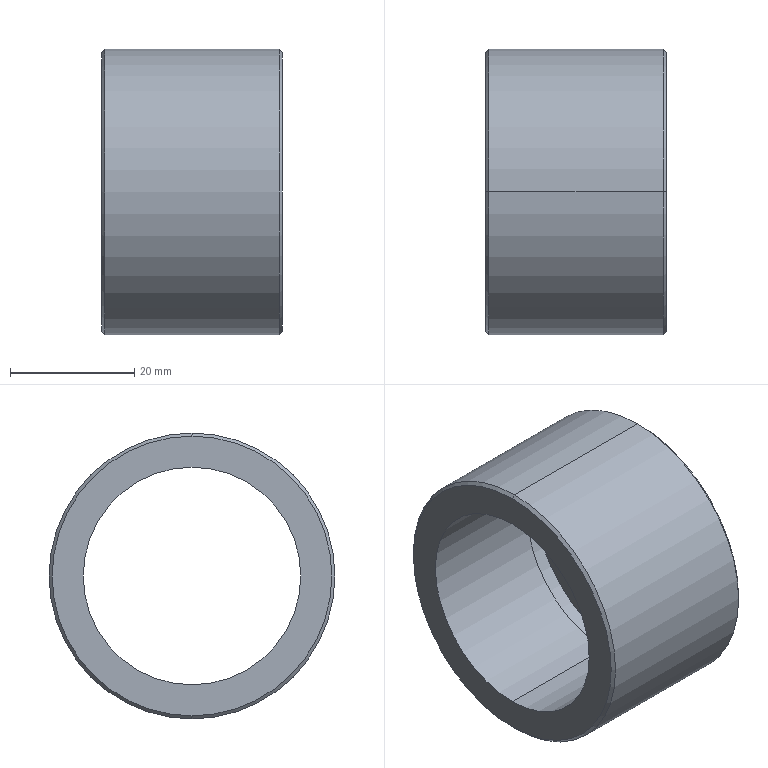Part | SolidWorks | features Chamfer 1, Revolution 1 | 1 solid | 16 faces | box 29 x 46 x 46 mm | volume 17975 mm3 | cylinder 8 | cone 4 | plane 4 | commonest cylinder face diameters 35 x4 42.5 x2 46 x2
STEP:
#1=CARTESIAN_POINT('',(0.,0.,22.5));
#2=VERTEX_POINT('',#1);
#3=CARTESIAN_POINT('',(0.,0.,-22.5));
#4=VERTEX_POINT('',#3);
#5=CARTESIAN_POINT('',(0.,0.,0.));
#6=DIRECTION('',(-1.,0.,0.));
#7=DIRECTION('',(0.,0.,-1.));
#8=AXIS2_PLACEMENT_3D('',#5,#6,#7);
#9=CIRCLE('',#8,22.5);
#10=EDGE_CURVE('',#2,#4,#9,.T.);
#11=ORIENTED_EDGE('',*,*,#10,.F.);
#12=CARTESIAN_POINT('',(0.5,0.,23.));
#13=VERTEX_POINT('',#12);
#14=CARTESIAN_POINT('',(0.,0.,22.5));
#15=DIRECTION('',(0.7071,0.,0.7071));
#16=VECTOR('',#15,1000.);
#17=LINE('',#14,#16);
#18=EDGE_CURVE('',#2,#13,#17,.T.);
#19=ORIENTED_EDGE('',*,*,#18,.T.);
#20=CARTESIAN_POINT('',(0.5,0.,-23.));
#21=VERTEX_POINT('',#20);
#22=CARTESIAN_POINT('',(0.5,0.,0.));
#23=DIRECTION('',(1.,0.,0.));
#24=DIRECTION('',(0.,0.,-1.));
#25=AXIS2_PLACEMENT_3D('',#22,#23,#24);
#26=CIRCLE('',#25,23.);
#27=EDGE_CURVE('',#21,#13,#26,.T.);
#28=ORIENTED_EDGE('',*,*,#27,.F.);
#29=CARTESIAN_POINT('',(0.,0.,-22.5));
#30=DIRECTION('',(0.7071,0.,-0.7071));
#31=VECTOR('',#30,1000.);
#32=LINE('',#29,#31);
#33=EDGE_CURVE('',#4,#21,#32,.T.);
#34=ORIENTED_EDGE('',*,*,#33,.F.);
#35=EDGE_LOOP('',(#11,#19,#28,#34));
#36=FACE_OUTER_BOUND('',#35,.T.);
#37=CARTESIAN_POINT('',(0.,0.,0.));
#38=DIRECTION('',(1.,0.,0.));
#39=DIRECTION('',(0.,0.,-1.));
#40=AXIS2_PLACEMENT_3D('',#37,#38,#39);
#41=CONICAL_SURFACE('',#40,22.5,0.7854);
#42=ADVANCED_FACE('',(#36),#41,.T.);
#43=CARTESIAN_POINT('',(29.,0.,-22.5));
#44=VERTEX_POINT('',#43);
#45=CARTESIAN_POINT('',(29.,0.,22.5));
#46=VERTEX_POINT('',#45);
#47=CARTESIAN_POINT('',(29.,0.,0.));
#48=DIRECTION('',(1.,0.,0.));
#49=DIRECTION('',(0.,0.,1.));
#50=AXIS2_PLACEMENT_3D('',#47,#48,#49);
#51=CIRCLE('',#50,22.5);
#52=EDGE_CURVE('',#44,#46,#51,.T.);
#53=ORIENTED_EDGE('',*,*,#52,.F.);
#54=CARTESIAN_POINT('',(28.5,0.,-23.));
#55=VERTEX_POINT('',#54);
#56=CARTESIAN_POINT('',(28.5,0.,-23.));
#57=DIRECTION('',(-0.7071,0.,-0.7071));
#58=VECTOR('',#57,1000.);
#59=LINE('',#56,#58);
#60=EDGE_CURVE('',#44,#55,#59,.T.);
#61=ORIENTED_EDGE('',*,*,#60,.T.);
#62=CARTESIAN_POINT('',(28.5,0.,23.));
#63=VERTEX_POINT('',#62);
#64=CARTESIAN_POINT('',(28.5,0.,0.));
#65=DIRECTION('',(-1.,0.,0.));
#66=DIRECTION('',(0.,0.,1.));
#67=AXIS2_PLACEMENT_3D('',#64,#65,#66);
#68=CIRCLE('',#67,23.);
#69=EDGE_CURVE('',#63,#55,#68,.T.);
#70=ORIENTED_EDGE('',*,*,#69,.F.);
#71=CARTESIAN_POINT('',(28.5,0.,23.));
#72=DIRECTION('',(-0.7071,0.,0.7071));
#73=VECTOR('',#72,1000.);
#74=LINE('',#71,#73);
#75=EDGE_CURVE('',#46,#63,#74,.T.);
#76=ORIENTED_EDGE('',*,*,#75,.F.);
#77=EDGE_LOOP('',(#53,#61,#70,#76));
#78=FACE_OUTER_BOUND('',#77,.T.);
#79=CARTESIAN_POINT('',(28.5,0.,0.));
#80=DIRECTION('',(-1.,0.,0.));
#81=DIRECTION('',(0.,0.,1.));
#82=AXIS2_PLACEMENT_3D('',#79,#80,#81);
#83=CONICAL_SURFACE('',#82,23.,0.7854);
#84=ADVANCED_FACE('',(#78),#83,.T.);
#85=CARTESIAN_POINT('',(21.,0.,-17.5));
#86=VERTEX_POINT('',#85);
#87=CARTESIAN_POINT('',(21.,0.,17.5));
#88=VERTEX_POINT('',#87);
#89=CARTESIAN_POINT('',(21.,0.,0.));
#90=DIRECTION('',(-1.,0.,0.));
#91=DIRECTION('',(0.,0.,1.));
#92=AXIS2_PLACEMENT_3D('',#89,#90,#91);
#93=CIRCLE('',#92,17.5);
#94=EDGE_CURVE('',#86,#88,#93,.T.);
#95=ORIENTED_EDGE('',*,*,#94,.F.);
#96=CARTESIAN_POINT('',(0.,0.,-17.5));
#97=VERTEX_POINT('',#96);
#98=CARTESIAN_POINT('',(0.,0.,-17.5));
#99=DIRECTION('',(-1.,0.,0.));
#100=VECTOR('',#99,1000.);
#101=LINE('',#98,#100);
#102=EDGE_CURVE('',#86,#97,#101,.T.);
#103=ORIENTED_EDGE('',*,*,#102,.T.);
#104=CARTESIAN_POINT('',(0.,0.,17.5));
#105=VERTEX_POINT('',#104);
#106=CARTESIAN_POINT('',(0.,0.,0.));
#107=DIRECTION('',(-1.,0.,0.));
#108=DIRECTION('',(0.,0.,1.));
#109=AXIS2_PLACEMENT_3D('',#106,#107,#108);
#110=CIRCLE('',#109,17.5);
#111=EDGE_CURVE('',#97,#105,#110,.T.);
#112=ORIENTED_EDGE('',*,*,#111,.T.);
#113=CARTESIAN_POINT('',(0.,0.,17.5));
#114=DIRECTION('',(-1.,0.,0.));
#115=VECTOR('',#114,1000.);
#116=LINE('',#113,#115);
#117=EDGE_CURVE('',#88,#105,#116,.T.);
#118=ORIENTED_EDGE('',*,*,#117,.F.);
#119=EDGE_LOOP('',(#95,#103,#112,#118));
#120=FACE_OUTER_BOUND('',#119,.T.);
#121=CARTESIAN_POINT('',(0.,0.,0.));
#122=DIRECTION('',(-1.,0.,0.));
#123=DIRECTION('',(0.,0.,1.));
#124=AXIS2_PLACEMENT_3D('',#121,#122,#123);
#125=CYLINDRICAL_SURFACE('',#124,17.5);
#126=ADVANCED_FACE('',(#120),#125,.F.);
#127=CARTESIAN_POINT('',(26.,0.,-21.25));
#128=VERTEX_POINT('',#127);
#129=CARTESIAN_POINT('',(26.,0.,21.25));
#130=VERTEX_POINT('',#129);
#131=CARTESIAN_POINT('',(26.,0.,0.));
#132=DIRECTION('',(-1.,0.,0.));
#133=DIRECTION('',(0.,0.,1.));
#134=AXIS2_PLACEMENT_3D('',#131,#132,#133);
#135=CIRCLE('',#134,21.25);
#136=EDGE_CURVE('',#128,#130,#135,.T.);
#137=ORIENTED_EDGE('',*,*,#136,.F.);
#138=CARTESIAN_POINT('',(21.,0.,-21.25));
#139=VERTEX_POINT('',#138);
#140=CARTESIAN_POINT('',(0.,0.,-21.25));
#141=DIRECTION('',(-1.,0.,0.));
#142=VECTOR('',#141,1000.);
#143=LINE('',#140,#142);
#144=EDGE_CURVE('',#128,#139,#143,.T.);
#145=ORIENTED_EDGE('',*,*,#144,.T.);
#146=CARTESIAN_POINT('',(21.,0.,21.25));
#147=VERTEX_POINT('',#146);
#148=CARTESIAN_POINT('',(21.,0.,0.));
#149=DIRECTION('',(-1.,0.,0.));
#150=DIRECTION('',(0.,0.,1.));
#151=AXIS2_PLACEMENT_3D('',#148,#149,#150);
#152=CIRCLE('',#151,21.25);
#153=EDGE_CURVE('',#139,#147,#152,.T.);
#154=ORIENTED_EDGE('',*,*,#153,.T.);
#155=CARTESIAN_POINT('',(0.,0.,21.25));
#156=DIRECTION('',(-1.,0.,0.));
#157=VECTOR('',#156,1000.);
#158=LINE('',#155,#157);
#159=EDGE_CURVE('',#130,#147,#158,.T.);
#160=ORIENTED_EDGE('',*,*,#159,.F.);
#161=EDGE_LOOP('',(#137,#145,#154,#160));
#162=FACE_OUTER_BOUND('',#161,.T.);
#163=CARTESIAN_POINT('',(0.,0.,0.));
#164=DIRECTION('',(-1.,0.,0.));
#165=DIRECTION('',(0.,0.,1.));
#166=AXIS2_PLACEMENT_3D('',#163,#164,#165);
#167=CYLINDRICAL_SURFACE('',#166,21.25);
#168=ADVANCED_FACE('',(#162),#167,.F.);
#169=CARTESIAN_POINT('',(29.,0.,-17.5));
#170=VERTEX_POINT('',#169);
#171=CARTESIAN_POINT('',(29.,0.,17.5));
#172=VERTEX_POINT('',#171);
#173=CARTESIAN_POINT('',(29.,0.,0.));
#174=DIRECTION('',(-1.,0.,0.));
#175=DIRECTION('',(0.,0.,1.));
#176=AXIS2_PLACEMENT_3D('',#173,#174,#175);
#177=CIRCLE('',#176,17.5);
#178=EDGE_CURVE('',#170,#172,#177,.T.);
#179=ORIENTED_EDGE('',*,*,#178,.F.);
#180=CARTESIAN_POINT('',(26.,0.,-17.5));
#181=VERTEX_POINT('',#180);
#182=CARTESIAN_POINT('',(0.,0.,-17.5));
#183=DIRECTION('',(-1.,0.,0.));
#184=VECTOR('',#183,1000.);
#185=LINE('',#182,#184);
#186=EDGE_CURVE('',#170,#181,#185,.T.);
#187=ORIENTED_EDGE('',*,*,#186,.T.);
#188=CARTESIAN_POINT('',(26.,0.,17.5));
#189=VERTEX_POINT('',#188);
#190=CARTESIAN_POINT('',(26.,0.,0.));
#191=DIRECTION('',(-1.,0.,0.));
#192=DIRECTION('',(0.,0.,1.));
#193=AXIS2_PLACEMENT_3D('',#190,#191,#192);
#194=CIRCLE('',#193,17.5);
#195=EDGE_CURVE('',#181,#189,#194,.T.);
#196=ORIENTED_EDGE('',*,*,#195,.T.);
#197=CARTESIAN_POINT('',(0.,0.,17.5));
#198=DIRECTION('',(-1.,0.,0.));
#199=VECTOR('',#198,1000.);
#200=LINE('',#197,#199);
#201=EDGE_CURVE('',#172,#189,#200,.T.);
#202=ORIENTED_EDGE('',*,*,#201,.F.);
#203=EDGE_LOOP('',(#179,#187,#196,#202));
#204=FACE_OUTER_BOUND('',#203,.T.);
#205=CARTESIAN_POINT('',(0.,0.,0.));
#206=DIRECTION('',(-1.,0.,0.));
#207=DIRECTION('',(0.,0.,1.));
#208=AXIS2_PLACEMENT_3D('',#205,#206,#207);
#209=CYLINDRICAL_SURFACE('',#208,17.5);
#210=ADVANCED_FACE('',(#204),#209,.F.);
#211=ORIENTED_EDGE('',*,*,#69,.T.);
#212=CARTESIAN_POINT('',(0.,0.,-23.));
#213=DIRECTION('',(-1.,0.,0.));
#214=VECTOR('',#213,1000.);
#215=LINE('',#212,#214);
#216=EDGE_CURVE('',#55,#21,#215,.T.);
#217=ORIENTED_EDGE('',*,*,#216,.T.);
#218=ORIENTED_EDGE('',*,*,#27,.T.);
#219=CARTESIAN_POINT('',(0.,0.,23.));
#220=DIRECTION('',(-1.,0.,0.));
#221=VECTOR('',#220,1000.);
#222=LINE('',#219,#221);
#223=EDGE_CURVE('',#63,#13,#222,.T.);
#224=ORIENTED_EDGE('',*,*,#223,.F.);
#225=EDGE_LOOP('',(#211,#217,#218,#224));
#226=FACE_OUTER_BOUND('',#225,.T.);
#227=CARTESIAN_POINT('',(0.,0.,0.));
#228=DIRECTION('',(-1.,0.,0.));
#229=DIRECTION('',(0.,0.,1.));
#230=AXIS2_PLACEMENT_3D('',#227,#228,#229);
#231=CYLINDRICAL_SURFACE('',#230,23.);
#232=ADVANCED_FACE('',(#226),#231,.T.);
#233=CARTESIAN_POINT('',(0.,0.,0.));
#234=DIRECTION('',(-1.,0.,0.));
#235=DIRECTION('',(0.,0.,-1.));
#236=AXIS2_PLACEMENT_3D('',#233,#234,#235);
#237=CIRCLE('',#236,22.5);
#238=EDGE_CURVE('',#4,#2,#237,.T.);
#239=ORIENTED_EDGE('',*,*,#238,.T.);
#240=ORIENTED_EDGE('',*,*,#10,.T.);
#241=EDGE_LOOP('',(#239,#240));
#242=FACE_OUTER_BOUND('',#241,.T.);
#243=CARTESIAN_POINT('',(0.,0.,0.));
#244=DIRECTION('',(-1.,0.,0.));
#245=DIRECTION('',(0.,0.,1.));
#246=AXIS2_PLACEMENT_3D('',#243,#244,#245);
#247=CIRCLE('',#246,17.5);
#248=EDGE_CURVE('',#105,#97,#247,.T.);
#249=ORIENTED_EDGE('',*,*,#248,.F.);
#250=ORIENTED_EDGE('',*,*,#111,.F.);
#251=EDGE_LOOP('',(#249,#250));
#252=FACE_BOUND('',#251,.T.);
#253=CARTESIAN_POINT('',(0.,17.5,0.));
#254=DIRECTION('',(1.,0.,0.));
#255=DIRECTION('',(0.,0.,-1.));
#256=AXIS2_PLACEMENT_3D('',#253,#254,#255);
#257=PLANE('',#256);
#258=ADVANCED_FACE('',(#242,#252),#257,.F.);
#259=ORIENTED_EDGE('',*,*,#216,.F.);
#260=CARTESIAN_POINT('',(28.5,0.,0.));
#261=DIRECTION('',(-1.,0.,0.));
#262=DIRECTION('',(0.,0.,1.));
#263=AXIS2_PLACEMENT_3D('',#260,#261,#262);
#264=CIRCLE('',#263,23.);
#265=EDGE_CURVE('',#55,#63,#264,.T.);
#266=ORIENTED_EDGE('',*,*,#265,.T.);
#267=ORIENTED_EDGE('',*,*,#223,.T.);
#268=CARTESIAN_POINT('',(0.5,0.,0.));
#269=DIRECTION('',(1.,0.,0.));
#270=DIRECTION('',(0.,0.,-1.));
#271=AXIS2_PLACEMENT_3D('',#268,#269,#270);
#272=CIRCLE('',#271,23.);
#273=EDGE_CURVE('',#13,#21,#272,.T.);
#274=ORIENTED_EDGE('',*,*,#273,.T.);
#275=EDGE_LOOP('',(#259,#266,#267,#274));
#276=FACE_OUTER_BOUND('',#275,.T.);
#277=CARTESIAN_POINT('',(0.,0.,0.));
#278=DIRECTION('',(-1.,0.,0.));
#279=DIRECTION('',(0.,0.,1.));
#280=AXIS2_PLACEMENT_3D('',#277,#278,#279);
#281=CYLINDRICAL_SURFACE('',#280,23.);
#282=ADVANCED_FACE('',(#276),#281,.T.);
#283=CARTESIAN_POINT('',(29.,0.,0.));
#284=DIRECTION('',(1.,0.,0.));
#285=DIRECTION('',(0.,0.,1.));
#286=AXIS2_PLACEMENT_3D('',#283,#284,#285);
#287=CIRCLE('',#286,22.5);
#288=EDGE_CURVE('',#46,#44,#287,.T.);
#289=ORIENTED_EDGE('',*,*,#288,.T.);
#290=ORIENTED_EDGE('',*,*,#52,.T.);
#291=EDGE_LOOP('',(#289,#290));
#292=FACE_OUTER_BOUND('',#291,.T.);
#293=CARTESIAN_POINT('',(29.,0.,0.));
#294=DIRECTION('',(-1.,0.,0.));
#295=DIRECTION('',(0.,0.,1.));
#296=AXIS2_PLACEMENT_3D('',#293,#294,#295);
#297=CIRCLE('',#296,17.5);
#298=EDGE_CURVE('',#172,#170,#297,.T.);
#299=ORIENTED_EDGE('',*,*,#298,.T.);
#300=ORIENTED_EDGE('',*,*,#178,.T.);
#301=EDGE_LOOP('',(#299,#300));
#302=FACE_BOUND('',#301,.T.);
#303=CARTESIAN_POINT('',(29.,17.5,0.));
#304=DIRECTION('',(-1.,0.,0.));
#305=DIRECTION('',(0.,0.,1.));
#306=AXIS2_PLACEMENT_3D('',#303,#304,#305);
#307=PLANE('',#306);
#308=ADVANCED_FACE('',(#292,#302),#307,.F.);
#309=ORIENTED_EDGE('',*,*,#186,.F.);
#310=ORIENTED_EDGE('',*,*,#298,.F.);
#311=ORIENTED_EDGE('',*,*,#201,.T.);
#312=CARTESIAN_POINT('',(26.,0.,0.));
#313=DIRECTION('',(-1.,0.,0.));
#314=DIRECTION('',(0.,0.,1.));
#315=AXIS2_PLACEMENT_3D('',#312,#313,#314);
#316=CIRCLE('',#315,17.5);
#317=EDGE_CURVE('',#189,#181,#316,.T.);
#318=ORIENTED_EDGE('',*,*,#317,.T.);
#319=EDGE_LOOP('',(#309,#310,#311,#318));
#320=FACE_OUTER_BOUND('',#319,.T.);
#321=CARTESIAN_POINT('',(0.,0.,0.));
#322=DIRECTION('',(-1.,0.,0.));
#323=DIRECTION('',(0.,0.,1.));
#324=AXIS2_PLACEMENT_3D('',#321,#322,#323);
#325=CYLINDRICAL_SURFACE('',#324,17.5);
#326=ADVANCED_FACE('',(#320),#325,.F.);
#327=ORIENTED_EDGE('',*,*,#317,.F.);
#328=ORIENTED_EDGE('',*,*,#195,.F.);
#329=EDGE_LOOP('',(#327,#328));
#330=FACE_BOUND('',#329,.T.);
#331=CARTESIAN_POINT('',(26.,0.,0.));
#332=DIRECTION('',(-1.,0.,0.));
#333=DIRECTION('',(0.,0.,1.));
#334=AXIS2_PLACEMENT_3D('',#331,#332,#333);
#335=CIRCLE('',#334,21.25);
#336=EDGE_CURVE('',#130,#128,#335,.T.);
#337=ORIENTED_EDGE('',*,*,#336,.T.);
#338=ORIENTED_EDGE('',*,*,#136,.T.);
#339=EDGE_LOOP('',(#337,#338));
#340=FACE_OUTER_BOUND('',#339,.T.);
#341=CARTESIAN_POINT('',(26.,21.25,0.));
#342=DIRECTION('',(1.,0.,0.));
#343=DIRECTION('',(0.,0.,-1.));
#344=AXIS2_PLACEMENT_3D('',#341,#342,#343);
#345=PLANE('',#344);
#346=ADVANCED_FACE('',(#330,#340),#345,.F.);
#347=ORIENTED_EDGE('',*,*,#144,.F.);
#348=ORIENTED_EDGE('',*,*,#336,.F.);
#349=ORIENTED_EDGE('',*,*,#159,.T.);
#350=CARTESIAN_POINT('',(21.,0.,0.));
#351=DIRECTION('',(-1.,0.,0.));
#352=DIRECTION('',(0.,0.,1.));
#353=AXIS2_PLACEMENT_3D('',#350,#351,#352);
#354=CIRCLE('',#353,21.25);
#355=EDGE_CURVE('',#147,#139,#354,.T.);
#356=ORIENTED_EDGE('',*,*,#355,.T.);
#357=EDGE_LOOP('',(#347,#348,#349,#356));
#358=FACE_OUTER_BOUND('',#357,.T.);
#359=CARTESIAN_POINT('',(0.,0.,0.));
#360=DIRECTION('',(-1.,0.,0.));
#361=DIRECTION('',(0.,0.,1.));
#362=AXIS2_PLACEMENT_3D('',#359,#360,#361);
#363=CYLINDRICAL_SURFACE('',#362,21.25);
#364=ADVANCED_FACE('',(#358),#363,.F.);
#365=ORIENTED_EDGE('',*,*,#355,.F.);
#366=ORIENTED_EDGE('',*,*,#153,.F.);
#367=EDGE_LOOP('',(#365,#366));
#368=FACE_OUTER_BOUND('',#367,.T.);
#369=CARTESIAN_POINT('',(21.,0.,0.));
#370=DIRECTION('',(-1.,0.,0.));
#371=DIRECTION('',(0.,0.,1.));
#372=AXIS2_PLACEMENT_3D('',#369,#370,#371);
#373=CIRCLE('',#372,17.5);
#374=EDGE_CURVE('',#88,#86,#373,.T.);
#375=ORIENTED_EDGE('',*,*,#374,.T.);
#376=ORIENTED_EDGE('',*,*,#94,.T.);
#377=EDGE_LOOP('',(#375,#376));
#378=FACE_BOUND('',#377,.T.);
#379=CARTESIAN_POINT('',(21.,17.5,0.));
#380=DIRECTION('',(-1.,0.,0.));
#381=DIRECTION('',(0.,0.,1.));
#382=AXIS2_PLACEMENT_3D('',#379,#380,#381);
#383=PLANE('',#382);
#384=ADVANCED_FACE('',(#368,#378),#383,.F.);
#385=ORIENTED_EDGE('',*,*,#102,.F.);
#386=ORIENTED_EDGE('',*,*,#374,.F.);
#387=ORIENTED_EDGE('',*,*,#117,.T.);
#388=ORIENTED_EDGE('',*,*,#248,.T.);
#389=EDGE_LOOP('',(#385,#386,#387,#388));
#390=FACE_OUTER_BOUND('',#389,.T.);
#391=CARTESIAN_POINT('',(0.,0.,0.));
#392=DIRECTION('',(-1.,0.,0.));
#393=DIRECTION('',(0.,0.,1.));
#394=AXIS2_PLACEMENT_3D('',#391,#392,#393);
#395=CYLINDRICAL_SURFACE('',#394,17.5);
#396=ADVANCED_FACE('',(#390),#395,.F.);
#397=ORIENTED_EDGE('',*,*,#60,.F.);
#398=ORIENTED_EDGE('',*,*,#288,.F.);
#399=ORIENTED_EDGE('',*,*,#75,.T.);
#400=ORIENTED_EDGE('',*,*,#265,.F.);
#401=EDGE_LOOP('',(#397,#398,#399,#400));
#402=FACE_OUTER_BOUND('',#401,.T.);
#403=CARTESIAN_POINT('',(28.5,0.,0.));
#404=DIRECTION('',(-1.,0.,0.));
#405=DIRECTION('',(0.,0.,1.));
#406=AXIS2_PLACEMENT_3D('',#403,#404,#405);
#407=CONICAL_SURFACE('',#406,23.,0.7854);
#408=ADVANCED_FACE('',(#402),#407,.T.);
#409=ORIENTED_EDGE('',*,*,#18,.F.);
#410=ORIENTED_EDGE('',*,*,#238,.F.);
#411=ORIENTED_EDGE('',*,*,#33,.T.);
#412=ORIENTED_EDGE('',*,*,#273,.F.);
#413=EDGE_LOOP('',(#409,#410,#411,#412));
#414=FACE_OUTER_BOUND('',#413,.T.);
#415=CARTESIAN_POINT('',(0.,0.,0.));
#416=DIRECTION('',(1.,0.,0.));
#417=DIRECTION('',(0.,0.,-1.));
#418=AXIS2_PLACEMENT_3D('',#415,#416,#417);
#419=CONICAL_SURFACE('',#418,22.5,0.7854);
#420=ADVANCED_FACE('',(#414),#419,.T.);
#421=CLOSED_SHELL('',(#42,#84,#126,#168,#210,#232,#258,#282,#308,#326,#346,#364,#384,#396,#408,#420));
#422=MANIFOLD_SOLID_BREP('',#421);
#423=CARTESIAN_POINT('',(0.,0.,0.));
#424=DIRECTION('',(0.,0.,1.));
#425=DIRECTION('',(1.,0.,0.));
#426=AXIS2_PLACEMENT_3D('',#423,#424,#425);
#427=(LENGTH_UNIT()NAMED_UNIT(*)SI_UNIT(.MILLI.,.METRE.));
#428=UNCERTAINTY_MEASURE_WITH_UNIT(LENGTH_MEASURE(0.00001),#427,'','');
#429=(NAMED_UNIT(*)PLANE_ANGLE_UNIT()SI_UNIT($,.RADIAN.));
#430=(NAMED_UNIT(*)SI_UNIT($,.STERADIAN.)SOLID_ANGLE_UNIT());
#431=(GEOMETRIC_REPRESENTATION_CONTEXT(3)GLOBAL_UNCERTAINTY_ASSIGNED_CONTEXT((#428))GLOBAL_UNIT_ASSIGNED_CONTEXT((#427,#429,#430))REPRESENTATION_CONTEXT('',''));
#432=ADVANCED_BREP_SHAPE_REPRESENTATION('',(#422,#426),#431);